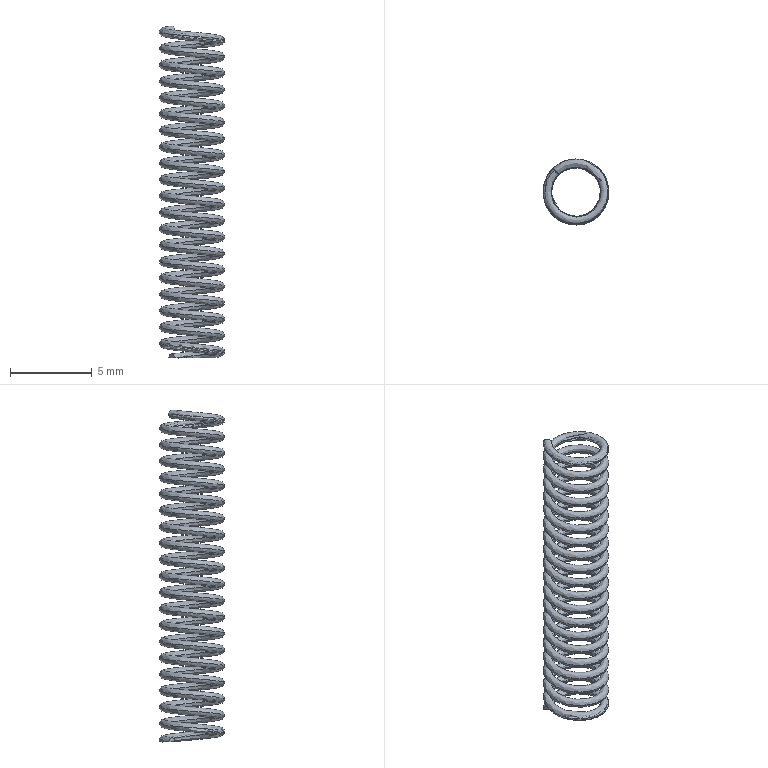Part | STEP file | spring-1 | 1 solid | 5 faces | box 3.998 x 3.998 x 20.249 mm | volume 43.124 mm3 | plane 3 | spline 2